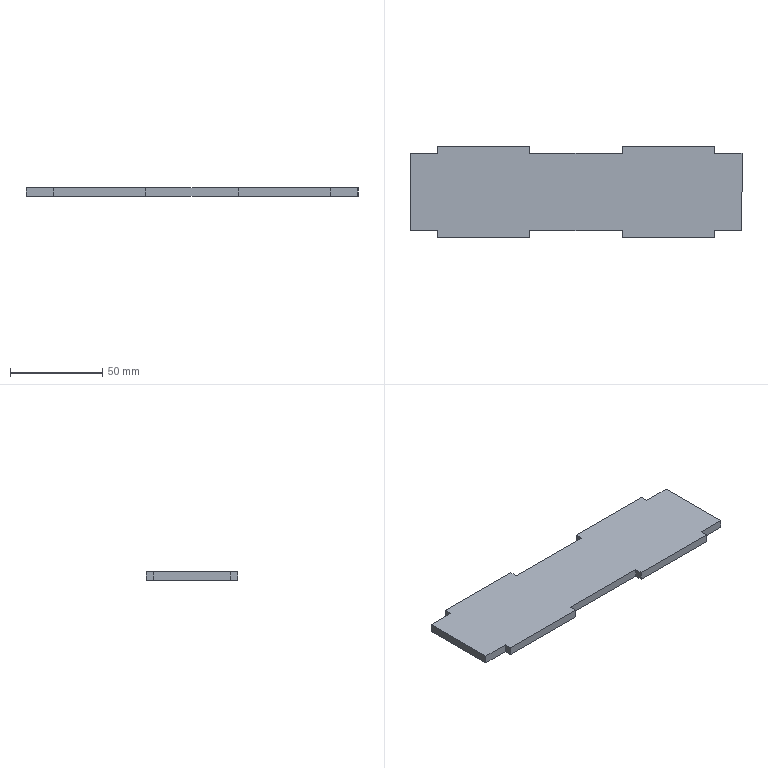Part | SolidWorks | features FlatPattern 1, SMBaseFlange 1, SheetMetal 1 | 1 solid | 22 faces | box 180 x 49.8 x 4.5 mm | volume 37458 mm3 | plane 22
STEP:
#1=CARTESIAN_POINT('',(68.167,-1112.571,0.));
#2=VERTEX_POINT('',#1);
#3=CARTESIAN_POINT('',(53.167,-1112.571,0.));
#4=VERTEX_POINT('',#3);
#5=CARTESIAN_POINT('',(53.167,-1112.571,0.));
#6=DIRECTION('',(-1.,0.,0.));
#7=VECTOR('',#6,1000.);
#8=LINE('',#5,#7);
#9=EDGE_CURVE('',#2,#4,#8,.T.);
#10=ORIENTED_EDGE('',*,*,#9,.F.);
#11=CARTESIAN_POINT('',(68.167,-1112.571,-4.5));
#12=VERTEX_POINT('',#11);
#13=CARTESIAN_POINT('',(68.167,-1112.571,-4.5));
#14=DIRECTION('',(0.,0.,1.));
#15=VECTOR('',#14,1000.);
#16=LINE('',#13,#15);
#17=EDGE_CURVE('',#12,#2,#16,.T.);
#18=ORIENTED_EDGE('',*,*,#17,.F.);
#19=CARTESIAN_POINT('',(53.167,-1112.571,-4.5));
#20=VERTEX_POINT('',#19);
#21=CARTESIAN_POINT('',(53.167,-1112.571,-4.5));
#22=DIRECTION('',(-1.,0.,0.));
#23=VECTOR('',#22,1000.);
#24=LINE('',#21,#23);
#25=EDGE_CURVE('',#12,#20,#24,.T.);
#26=ORIENTED_EDGE('',*,*,#25,.T.);
#27=CARTESIAN_POINT('',(53.167,-1112.571,-4.5));
#28=DIRECTION('',(0.,0.,1.));
#29=VECTOR('',#28,1000.);
#30=LINE('',#27,#29);
#31=EDGE_CURVE('',#20,#4,#30,.T.);
#32=ORIENTED_EDGE('',*,*,#31,.T.);
#33=EDGE_LOOP('',(#10,#18,#26,#32));
#34=FACE_OUTER_BOUND('',#33,.T.);
#35=CARTESIAN_POINT('',(53.167,-1112.571,-4.5));
#36=DIRECTION('',(0.,1.,0.));
#37=DIRECTION('',(0.,0.,1.));
#38=AXIS2_PLACEMENT_3D('',#35,#36,#37);
#39=PLANE('',#38);
#40=ADVANCED_FACE('',(#34),#39,.T.);
#41=CARTESIAN_POINT('',(68.167,-1154.371,0.));
#42=VERTEX_POINT('',#41);
#43=CARTESIAN_POINT('',(68.167,-1112.571,0.));
#44=DIRECTION('',(0.,1.,0.));
#45=VECTOR('',#44,1000.);
#46=LINE('',#43,#45);
#47=EDGE_CURVE('',#42,#2,#46,.T.);
#48=ORIENTED_EDGE('',*,*,#47,.F.);
#49=CARTESIAN_POINT('',(68.167,-1154.371,-4.5));
#50=VERTEX_POINT('',#49);
#51=CARTESIAN_POINT('',(68.167,-1154.371,-4.5));
#52=DIRECTION('',(0.,0.,1.));
#53=VECTOR('',#52,1000.);
#54=LINE('',#51,#53);
#55=EDGE_CURVE('',#50,#42,#54,.T.);
#56=ORIENTED_EDGE('',*,*,#55,.F.);
#57=CARTESIAN_POINT('',(68.167,-1112.571,-4.5));
#58=DIRECTION('',(0.,1.,0.));
#59=VECTOR('',#58,1000.);
#60=LINE('',#57,#59);
#61=EDGE_CURVE('',#50,#12,#60,.T.);
#62=ORIENTED_EDGE('',*,*,#61,.T.);
#63=ORIENTED_EDGE('',*,*,#17,.T.);
#64=EDGE_LOOP('',(#48,#56,#62,#63));
#65=FACE_OUTER_BOUND('',#64,.T.);
#66=CARTESIAN_POINT('',(68.167,-1112.571,-4.5));
#67=DIRECTION('',(1.,0.,0.));
#68=DIRECTION('',(0.,1.,0.));
#69=AXIS2_PLACEMENT_3D('',#66,#67,#68);
#70=PLANE('',#69);
#71=ADVANCED_FACE('',(#65),#70,.T.);
#72=CARTESIAN_POINT('',(53.167,-1154.371,0.));
#73=VERTEX_POINT('',#72);
#74=CARTESIAN_POINT('',(68.167,-1154.371,0.));
#75=DIRECTION('',(1.,0.,0.));
#76=VECTOR('',#75,1000.);
#77=LINE('',#74,#76);
#78=EDGE_CURVE('',#73,#42,#77,.T.);
#79=ORIENTED_EDGE('',*,*,#78,.F.);
#80=CARTESIAN_POINT('',(53.167,-1154.371,-4.5));
#81=VERTEX_POINT('',#80);
#82=CARTESIAN_POINT('',(53.167,-1154.371,-4.5));
#83=DIRECTION('',(0.,0.,1.));
#84=VECTOR('',#83,1000.);
#85=LINE('',#82,#84);
#86=EDGE_CURVE('',#81,#73,#85,.T.);
#87=ORIENTED_EDGE('',*,*,#86,.F.);
#88=CARTESIAN_POINT('',(68.167,-1154.371,-4.5));
#89=DIRECTION('',(1.,0.,0.));
#90=VECTOR('',#89,1000.);
#91=LINE('',#88,#90);
#92=EDGE_CURVE('',#81,#50,#91,.T.);
#93=ORIENTED_EDGE('',*,*,#92,.T.);
#94=ORIENTED_EDGE('',*,*,#55,.T.);
#95=EDGE_LOOP('',(#79,#87,#93,#94));
#96=FACE_OUTER_BOUND('',#95,.T.);
#97=CARTESIAN_POINT('',(68.167,-1154.371,-4.5));
#98=DIRECTION('',(0.,-1.,0.));
#99=DIRECTION('',(0.,0.,-1.));
#100=AXIS2_PLACEMENT_3D('',#97,#98,#99);
#101=PLANE('',#100);
#102=ADVANCED_FACE('',(#96),#101,.T.);
#103=CARTESIAN_POINT('',(53.167,-1158.371,0.));
#104=VERTEX_POINT('',#103);
#105=CARTESIAN_POINT('',(53.167,-1154.371,0.));
#106=DIRECTION('',(0.,1.,0.));
#107=VECTOR('',#106,1000.);
#108=LINE('',#105,#107);
#109=EDGE_CURVE('',#104,#73,#108,.T.);
#110=ORIENTED_EDGE('',*,*,#109,.F.);
#111=CARTESIAN_POINT('',(53.167,-1158.371,-4.5));
#112=VERTEX_POINT('',#111);
#113=CARTESIAN_POINT('',(53.167,-1158.371,-4.5));
#114=DIRECTION('',(0.,0.,1.));
#115=VECTOR('',#114,1000.);
#116=LINE('',#113,#115);
#117=EDGE_CURVE('',#112,#104,#116,.T.);
#118=ORIENTED_EDGE('',*,*,#117,.F.);
#119=CARTESIAN_POINT('',(53.167,-1154.371,-4.5));
#120=DIRECTION('',(0.,1.,0.));
#121=VECTOR('',#120,1000.);
#122=LINE('',#119,#121);
#123=EDGE_CURVE('',#112,#81,#122,.T.);
#124=ORIENTED_EDGE('',*,*,#123,.T.);
#125=ORIENTED_EDGE('',*,*,#86,.T.);
#126=EDGE_LOOP('',(#110,#118,#124,#125));
#127=FACE_OUTER_BOUND('',#126,.T.);
#128=CARTESIAN_POINT('',(53.167,-1154.371,-4.5));
#129=DIRECTION('',(1.,0.,0.));
#130=DIRECTION('',(0.,1.,0.));
#131=AXIS2_PLACEMENT_3D('',#128,#129,#130);
#132=PLANE('',#131);
#133=ADVANCED_FACE('',(#127),#132,.T.);
#134=CARTESIAN_POINT('',(3.167,-1158.371,0.));
#135=VERTEX_POINT('',#134);
#136=CARTESIAN_POINT('',(53.167,-1158.371,0.));
#137=DIRECTION('',(1.,0.,0.));
#138=VECTOR('',#137,1000.);
#139=LINE('',#136,#138);
#140=EDGE_CURVE('',#135,#104,#139,.T.);
#141=ORIENTED_EDGE('',*,*,#140,.F.);
#142=CARTESIAN_POINT('',(3.167,-1158.371,-4.5));
#143=VERTEX_POINT('',#142);
#144=CARTESIAN_POINT('',(3.167,-1158.371,-4.5));
#145=DIRECTION('',(0.,0.,1.));
#146=VECTOR('',#145,1000.);
#147=LINE('',#144,#146);
#148=EDGE_CURVE('',#143,#135,#147,.T.);
#149=ORIENTED_EDGE('',*,*,#148,.F.);
#150=CARTESIAN_POINT('',(53.167,-1158.371,-4.5));
#151=DIRECTION('',(1.,0.,0.));
#152=VECTOR('',#151,1000.);
#153=LINE('',#150,#152);
#154=EDGE_CURVE('',#143,#112,#153,.T.);
#155=ORIENTED_EDGE('',*,*,#154,.T.);
#156=ORIENTED_EDGE('',*,*,#117,.T.);
#157=EDGE_LOOP('',(#141,#149,#155,#156));
#158=FACE_OUTER_BOUND('',#157,.T.);
#159=CARTESIAN_POINT('',(53.167,-1158.371,-4.5));
#160=DIRECTION('',(0.,-1.,0.));
#161=DIRECTION('',(0.,0.,-1.));
#162=AXIS2_PLACEMENT_3D('',#159,#160,#161);
#163=PLANE('',#162);
#164=ADVANCED_FACE('',(#158),#163,.T.);
#165=CARTESIAN_POINT('',(3.167,-1154.371,0.));
#166=VERTEX_POINT('',#165);
#167=CARTESIAN_POINT('',(3.167,-1158.371,0.));
#168=DIRECTION('',(0.,-1.,0.));
#169=VECTOR('',#168,1000.);
#170=LINE('',#167,#169);
#171=EDGE_CURVE('',#166,#135,#170,.T.);
#172=ORIENTED_EDGE('',*,*,#171,.F.);
#173=CARTESIAN_POINT('',(3.167,-1154.371,-4.5));
#174=VERTEX_POINT('',#173);
#175=CARTESIAN_POINT('',(3.167,-1154.371,-4.5));
#176=DIRECTION('',(0.,0.,1.));
#177=VECTOR('',#176,1000.);
#178=LINE('',#175,#177);
#179=EDGE_CURVE('',#174,#166,#178,.T.);
#180=ORIENTED_EDGE('',*,*,#179,.F.);
#181=CARTESIAN_POINT('',(3.167,-1158.371,-4.5));
#182=DIRECTION('',(0.,-1.,0.));
#183=VECTOR('',#182,1000.);
#184=LINE('',#181,#183);
#185=EDGE_CURVE('',#174,#143,#184,.T.);
#186=ORIENTED_EDGE('',*,*,#185,.T.);
#187=ORIENTED_EDGE('',*,*,#148,.T.);
#188=EDGE_LOOP('',(#172,#180,#186,#187));
#189=FACE_OUTER_BOUND('',#188,.T.);
#190=CARTESIAN_POINT('',(3.167,-1158.371,-4.5));
#191=DIRECTION('',(-1.,0.,0.));
#192=DIRECTION('',(0.,-1.,0.));
#193=AXIS2_PLACEMENT_3D('',#190,#191,#192);
#194=PLANE('',#193);
#195=ADVANCED_FACE('',(#189),#194,.T.);
#196=CARTESIAN_POINT('',(-46.833,-1154.371,0.));
#197=VERTEX_POINT('',#196);
#198=CARTESIAN_POINT('',(3.167,-1154.371,0.));
#199=DIRECTION('',(1.,0.,0.));
#200=VECTOR('',#199,1000.);
#201=LINE('',#198,#200);
#202=EDGE_CURVE('',#197,#166,#201,.T.);
#203=ORIENTED_EDGE('',*,*,#202,.F.);
#204=CARTESIAN_POINT('',(-46.833,-1154.371,-4.5));
#205=VERTEX_POINT('',#204);
#206=CARTESIAN_POINT('',(-46.833,-1154.371,-4.5));
#207=DIRECTION('',(0.,0.,1.));
#208=VECTOR('',#207,1000.);
#209=LINE('',#206,#208);
#210=EDGE_CURVE('',#205,#197,#209,.T.);
#211=ORIENTED_EDGE('',*,*,#210,.F.);
#212=CARTESIAN_POINT('',(3.167,-1154.371,-4.5));
#213=DIRECTION('',(1.,0.,0.));
#214=VECTOR('',#213,1000.);
#215=LINE('',#212,#214);
#216=EDGE_CURVE('',#205,#174,#215,.T.);
#217=ORIENTED_EDGE('',*,*,#216,.T.);
#218=ORIENTED_EDGE('',*,*,#179,.T.);
#219=EDGE_LOOP('',(#203,#211,#217,#218));
#220=FACE_OUTER_BOUND('',#219,.T.);
#221=CARTESIAN_POINT('',(3.167,-1154.371,-4.5));
#222=DIRECTION('',(0.,-1.,0.));
#223=DIRECTION('',(0.,0.,-1.));
#224=AXIS2_PLACEMENT_3D('',#221,#222,#223);
#225=PLANE('',#224);
#226=ADVANCED_FACE('',(#220),#225,.T.);
#227=CARTESIAN_POINT('',(-46.833,-1158.371,0.));
#228=VERTEX_POINT('',#227);
#229=CARTESIAN_POINT('',(-46.833,-1154.371,0.));
#230=DIRECTION('',(0.,1.,0.));
#231=VECTOR('',#230,1000.);
#232=LINE('',#229,#231);
#233=EDGE_CURVE('',#228,#197,#232,.T.);
#234=ORIENTED_EDGE('',*,*,#233,.F.);
#235=CARTESIAN_POINT('',(-46.833,-1158.371,-4.5));
#236=VERTEX_POINT('',#235);
#237=CARTESIAN_POINT('',(-46.833,-1158.371,-4.5));
#238=DIRECTION('',(0.,0.,1.));
#239=VECTOR('',#238,1000.);
#240=LINE('',#237,#239);
#241=EDGE_CURVE('',#236,#228,#240,.T.);
#242=ORIENTED_EDGE('',*,*,#241,.F.);
#243=CARTESIAN_POINT('',(-46.833,-1154.371,-4.5));
#244=DIRECTION('',(0.,1.,0.));
#245=VECTOR('',#244,1000.);
#246=LINE('',#243,#245);
#247=EDGE_CURVE('',#236,#205,#246,.T.);
#248=ORIENTED_EDGE('',*,*,#247,.T.);
#249=ORIENTED_EDGE('',*,*,#210,.T.);
#250=EDGE_LOOP('',(#234,#242,#248,#249));
#251=FACE_OUTER_BOUND('',#250,.T.);
#252=CARTESIAN_POINT('',(-46.833,-1154.371,-4.5));
#253=DIRECTION('',(1.,0.,0.));
#254=DIRECTION('',(0.,0.,-1.));
#255=AXIS2_PLACEMENT_3D('',#252,#253,#254);
#256=PLANE('',#255);
#257=ADVANCED_FACE('',(#251),#256,.T.);
#258=CARTESIAN_POINT('',(-96.833,-1158.371,0.));
#259=VERTEX_POINT('',#258);
#260=CARTESIAN_POINT('',(-46.833,-1158.371,0.));
#261=DIRECTION('',(1.,0.,0.));
#262=VECTOR('',#261,1000.);
#263=LINE('',#260,#262);
#264=EDGE_CURVE('',#259,#228,#263,.T.);
#265=ORIENTED_EDGE('',*,*,#264,.F.);
#266=CARTESIAN_POINT('',(-96.833,-1158.371,-4.5));
#267=VERTEX_POINT('',#266);
#268=CARTESIAN_POINT('',(-96.833,-1158.371,-4.5));
#269=DIRECTION('',(0.,0.,1.));
#270=VECTOR('',#269,1000.);
#271=LINE('',#268,#270);
#272=EDGE_CURVE('',#267,#259,#271,.T.);
#273=ORIENTED_EDGE('',*,*,#272,.F.);
#274=CARTESIAN_POINT('',(-46.833,-1158.371,-4.5));
#275=DIRECTION('',(1.,0.,0.));
#276=VECTOR('',#275,1000.);
#277=LINE('',#274,#276);
#278=EDGE_CURVE('',#267,#236,#277,.T.);
#279=ORIENTED_EDGE('',*,*,#278,.T.);
#280=ORIENTED_EDGE('',*,*,#241,.T.);
#281=EDGE_LOOP('',(#265,#273,#279,#280));
#282=FACE_OUTER_BOUND('',#281,.T.);
#283=CARTESIAN_POINT('',(-46.833,-1158.371,-4.5));
#284=DIRECTION('',(0.,-1.,0.));
#285=DIRECTION('',(0.,0.,-1.));
#286=AXIS2_PLACEMENT_3D('',#283,#284,#285);
#287=PLANE('',#286);
#288=ADVANCED_FACE('',(#282),#287,.T.);
#289=CARTESIAN_POINT('',(-96.833,-1154.371,0.));
#290=VERTEX_POINT('',#289);
#291=CARTESIAN_POINT('',(-96.833,-1158.371,0.));
#292=DIRECTION('',(0.,-1.,0.));
#293=VECTOR('',#292,1000.);
#294=LINE('',#291,#293);
#295=EDGE_CURVE('',#290,#259,#294,.T.);
#296=ORIENTED_EDGE('',*,*,#295,.F.);
#297=CARTESIAN_POINT('',(-96.833,-1154.371,-4.5));
#298=VERTEX_POINT('',#297);
#299=CARTESIAN_POINT('',(-96.833,-1154.371,-4.5));
#300=DIRECTION('',(0.,0.,1.));
#301=VECTOR('',#300,1000.);
#302=LINE('',#299,#301);
#303=EDGE_CURVE('',#298,#290,#302,.T.);
#304=ORIENTED_EDGE('',*,*,#303,.F.);
#305=CARTESIAN_POINT('',(-96.833,-1158.371,-4.5));
#306=DIRECTION('',(0.,-1.,0.));
#307=VECTOR('',#306,1000.);
#308=LINE('',#305,#307);
#309=EDGE_CURVE('',#298,#267,#308,.T.);
#310=ORIENTED_EDGE('',*,*,#309,.T.);
#311=ORIENTED_EDGE('',*,*,#272,.T.);
#312=EDGE_LOOP('',(#296,#304,#310,#311));
#313=FACE_OUTER_BOUND('',#312,.T.);
#314=CARTESIAN_POINT('',(-96.833,-1158.371,-4.5));
#315=DIRECTION('',(-1.,0.,0.));
#316=DIRECTION('',(0.,0.,1.));
#317=AXIS2_PLACEMENT_3D('',#314,#315,#316);
#318=PLANE('',#317);
#319=ADVANCED_FACE('',(#313),#318,.T.);
#320=CARTESIAN_POINT('',(-111.833,-1154.371,0.));
#321=VERTEX_POINT('',#320);
#322=CARTESIAN_POINT('',(-96.833,-1154.371,0.));
#323=DIRECTION('',(1.,0.,0.));
#324=VECTOR('',#323,1000.);
#325=LINE('',#322,#324);
#326=EDGE_CURVE('',#321,#290,#325,.T.);
#327=ORIENTED_EDGE('',*,*,#326,.F.);
#328=CARTESIAN_POINT('',(-111.833,-1154.371,-4.5));
#329=VERTEX_POINT('',#328);
#330=CARTESIAN_POINT('',(-111.833,-1154.371,-4.5));
#331=DIRECTION('',(0.,0.,1.));
#332=VECTOR('',#331,1000.);
#333=LINE('',#330,#332);
#334=EDGE_CURVE('',#329,#321,#333,.T.);
#335=ORIENTED_EDGE('',*,*,#334,.F.);
#336=CARTESIAN_POINT('',(-96.833,-1154.371,-4.5));
#337=DIRECTION('',(1.,0.,0.));
#338=VECTOR('',#337,1000.);
#339=LINE('',#336,#338);
#340=EDGE_CURVE('',#329,#298,#339,.T.);
#341=ORIENTED_EDGE('',*,*,#340,.T.);
#342=ORIENTED_EDGE('',*,*,#303,.T.);
#343=EDGE_LOOP('',(#327,#335,#341,#342));
#344=FACE_OUTER_BOUND('',#343,.T.);
#345=CARTESIAN_POINT('',(-96.833,-1154.371,-4.5));
#346=DIRECTION('',(0.,-1.,0.));
#347=DIRECTION('',(0.,0.,-1.));
#348=AXIS2_PLACEMENT_3D('',#345,#346,#347);
#349=PLANE('',#348);
#350=ADVANCED_FACE('',(#344),#349,.T.);
#351=CARTESIAN_POINT('',(-111.833,-1112.571,0.));
#352=VERTEX_POINT('',#351);
#353=CARTESIAN_POINT('',(-111.833,-1154.371,0.));
#354=DIRECTION('',(0.,-1.,0.));
#355=VECTOR('',#354,1000.);
#356=LINE('',#353,#355);
#357=EDGE_CURVE('',#352,#321,#356,.T.);
#358=ORIENTED_EDGE('',*,*,#357,.F.);
#359=CARTESIAN_POINT('',(-111.833,-1112.571,-4.5));
#360=VERTEX_POINT('',#359);
#361=CARTESIAN_POINT('',(-111.833,-1112.571,-4.5));
#362=DIRECTION('',(0.,0.,1.));
#363=VECTOR('',#362,1000.);
#364=LINE('',#361,#363);
#365=EDGE_CURVE('',#360,#352,#364,.T.);
#366=ORIENTED_EDGE('',*,*,#365,.F.);
#367=CARTESIAN_POINT('',(-111.833,-1154.371,-4.5));
#368=DIRECTION('',(0.,-1.,0.));
#369=VECTOR('',#368,1000.);
#370=LINE('',#367,#369);
#371=EDGE_CURVE('',#360,#329,#370,.T.);
#372=ORIENTED_EDGE('',*,*,#371,.T.);
#373=ORIENTED_EDGE('',*,*,#334,.T.);
#374=EDGE_LOOP('',(#358,#366,#372,#373));
#375=FACE_OUTER_BOUND('',#374,.T.);
#376=CARTESIAN_POINT('',(-111.833,-1154.371,-4.5));
#377=DIRECTION('',(-1.,0.,0.));
#378=DIRECTION('',(0.,-1.,0.));
#379=AXIS2_PLACEMENT_3D('',#376,#377,#378);
#380=PLANE('',#379);
#381=ADVANCED_FACE('',(#375),#380,.T.);
#382=CARTESIAN_POINT('',(-96.833,-1112.571,0.));
#383=VERTEX_POINT('',#382);
#384=CARTESIAN_POINT('',(-111.833,-1112.571,0.));
#385=DIRECTION('',(-1.,0.,0.));
#386=VECTOR('',#385,1000.);
#387=LINE('',#384,#386);
#388=EDGE_CURVE('',#383,#352,#387,.T.);
#389=ORIENTED_EDGE('',*,*,#388,.F.);
#390=CARTESIAN_POINT('',(-96.833,-1112.571,-4.5));
#391=VERTEX_POINT('',#390);
#392=CARTESIAN_POINT('',(-96.833,-1112.571,-4.5));
#393=DIRECTION('',(0.,0.,1.));
#394=VECTOR('',#393,1000.);
#395=LINE('',#392,#394);
#396=EDGE_CURVE('',#391,#383,#395,.T.);
#397=ORIENTED_EDGE('',*,*,#396,.F.);
#398=CARTESIAN_POINT('',(-111.833,-1112.571,-4.5));
#399=DIRECTION('',(-1.,0.,0.));
#400=VECTOR('',#399,1000.);
#401=LINE('',#398,#400);
#402=EDGE_CURVE('',#391,#360,#401,.T.);
#403=ORIENTED_EDGE('',*,*,#402,.T.);
#404=ORIENTED_EDGE('',*,*,#365,.T.);
#405=EDGE_LOOP('',(#389,#397,#403,#404));
#406=FACE_OUTER_BOUND('',#405,.T.);
#407=CARTESIAN_POINT('',(-111.833,-1112.571,-4.5));
#408=DIRECTION('',(0.,1.,0.));
#409=DIRECTION('',(0.,0.,1.));
#410=AXIS2_PLACEMENT_3D('',#407,#408,#409);
#411=PLANE('',#410);
#412=ADVANCED_FACE('',(#406),#411,.T.);
#413=CARTESIAN_POINT('',(-96.833,-1108.571,0.));
#414=VERTEX_POINT('',#413);
#415=CARTESIAN_POINT('',(-96.833,-1112.571,0.));
#416=DIRECTION('',(0.,-1.,0.));
#417=VECTOR('',#416,1000.);
#418=LINE('',#415,#417);
#419=EDGE_CURVE('',#414,#383,#418,.T.);
#420=ORIENTED_EDGE('',*,*,#419,.F.);
#421=CARTESIAN_POINT('',(-96.833,-1108.571,-4.5));
#422=VERTEX_POINT('',#421);
#423=CARTESIAN_POINT('',(-96.833,-1108.571,-4.5));
#424=DIRECTION('',(0.,0.,1.));
#425=VECTOR('',#424,1000.);
#426=LINE('',#423,#425);
#427=EDGE_CURVE('',#422,#414,#426,.T.);
#428=ORIENTED_EDGE('',*,*,#427,.F.);
#429=CARTESIAN_POINT('',(-96.833,-1112.571,-4.5));
#430=DIRECTION('',(0.,-1.,0.));
#431=VECTOR('',#430,1000.);
#432=LINE('',#429,#431);
#433=EDGE_CURVE('',#422,#391,#432,.T.);
#434=ORIENTED_EDGE('',*,*,#433,.T.);
#435=ORIENTED_EDGE('',*,*,#396,.T.);
#436=EDGE_LOOP('',(#420,#428,#434,#435));
#437=FACE_OUTER_BOUND('',#436,.T.);
#438=CARTESIAN_POINT('',(-96.833,-1112.571,-4.5));
#439=DIRECTION('',(-1.,0.,0.));
#440=DIRECTION('',(0.,-1.,0.));
#441=AXIS2_PLACEMENT_3D('',#438,#439,#440);
#442=PLANE('',#441);
#443=ADVANCED_FACE('',(#437),#442,.T.);
#444=CARTESIAN_POINT('',(-46.833,-1108.571,0.));
#445=VERTEX_POINT('',#444);
#446=CARTESIAN_POINT('',(-96.833,-1108.571,0.));
#447=DIRECTION('',(-1.,0.,0.));
#448=VECTOR('',#447,1000.);
#449=LINE('',#446,#448);
#450=EDGE_CURVE('',#445,#414,#449,.T.);
#451=ORIENTED_EDGE('',*,*,#450,.F.);
#452=CARTESIAN_POINT('',(-46.833,-1108.571,-4.5));
#453=VERTEX_POINT('',#452);
#454=CARTESIAN_POINT('',(-46.833,-1108.571,-4.5));
#455=DIRECTION('',(0.,0.,1.));
#456=VECTOR('',#455,1000.);
#457=LINE('',#454,#456);
#458=EDGE_CURVE('',#453,#445,#457,.T.);
#459=ORIENTED_EDGE('',*,*,#458,.F.);
#460=CARTESIAN_POINT('',(-96.833,-1108.571,-4.5));
#461=DIRECTION('',(-1.,0.,0.));
#462=VECTOR('',#461,1000.);
#463=LINE('',#460,#462);
#464=EDGE_CURVE('',#453,#422,#463,.T.);
#465=ORIENTED_EDGE('',*,*,#464,.T.);
#466=ORIENTED_EDGE('',*,*,#427,.T.);
#467=EDGE_LOOP('',(#451,#459,#465,#466));
#468=FACE_OUTER_BOUND('',#467,.T.);
#469=CARTESIAN_POINT('',(-96.833,-1108.571,-4.5));
#470=DIRECTION('',(0.,1.,0.));
#471=DIRECTION('',(0.,0.,1.));
#472=AXIS2_PLACEMENT_3D('',#469,#470,#471);
#473=PLANE('',#472);
#474=ADVANCED_FACE('',(#468),#473,.T.);
#475=CARTESIAN_POINT('',(-46.833,-1112.571,0.));
#476=VERTEX_POINT('',#475);
#477=CARTESIAN_POINT('',(-46.833,-1108.571,0.));
#478=DIRECTION('',(0.,1.,0.));
#479=VECTOR('',#478,1000.);
#480=LINE('',#477,#479);
#481=EDGE_CURVE('',#476,#445,#480,.T.);
#482=ORIENTED_EDGE('',*,*,#481,.F.);
#483=CARTESIAN_POINT('',(-46.833,-1112.571,-4.5));
#484=VERTEX_POINT('',#483);
#485=CARTESIAN_POINT('',(-46.833,-1112.571,-4.5));
#486=DIRECTION('',(0.,0.,1.));
#487=VECTOR('',#486,1000.);
#488=LINE('',#485,#487);
#489=EDGE_CURVE('',#484,#476,#488,.T.);
#490=ORIENTED_EDGE('',*,*,#489,.F.);
#491=CARTESIAN_POINT('',(-46.833,-1108.571,-4.5));
#492=DIRECTION('',(0.,1.,0.));
#493=VECTOR('',#492,1000.);
#494=LINE('',#491,#493);
#495=EDGE_CURVE('',#484,#453,#494,.T.);
#496=ORIENTED_EDGE('',*,*,#495,.T.);
#497=ORIENTED_EDGE('',*,*,#458,.T.);
#498=EDGE_LOOP('',(#482,#490,#496,#497));
#499=FACE_OUTER_BOUND('',#498,.T.);
#500=CARTESIAN_POINT('',(-46.833,-1108.571,-4.5));
#501=DIRECTION('',(1.,0.,0.));
#502=DIRECTION('',(0.,1.,0.));
#503=AXIS2_PLACEMENT_3D('',#500,#501,#502);
#504=PLANE('',#503);
#505=ADVANCED_FACE('',(#499),#504,.T.);
#506=CARTESIAN_POINT('',(3.167,-1112.571,0.));
#507=VERTEX_POINT('',#506);
#508=CARTESIAN_POINT('',(-46.833,-1112.571,0.));
#509=DIRECTION('',(-1.,0.,0.));
#510=VECTOR('',#509,1000.);
#511=LINE('',#508,#510);
#512=EDGE_CURVE('',#507,#476,#511,.T.);
#513=ORIENTED_EDGE('',*,*,#512,.F.);
#514=CARTESIAN_POINT('',(3.167,-1112.571,-4.5));
#515=VERTEX_POINT('',#514);
#516=CARTESIAN_POINT('',(3.167,-1112.571,-4.5));
#517=DIRECTION('',(0.,0.,1.));
#518=VECTOR('',#517,1000.);
#519=LINE('',#516,#518);
#520=EDGE_CURVE('',#515,#507,#519,.T.);
#521=ORIENTED_EDGE('',*,*,#520,.F.);
#522=CARTESIAN_POINT('',(-46.833,-1112.571,-4.5));
#523=DIRECTION('',(-1.,0.,0.));
#524=VECTOR('',#523,1000.);
#525=LINE('',#522,#524);
#526=EDGE_CURVE('',#515,#484,#525,.T.);
#527=ORIENTED_EDGE('',*,*,#526,.T.);
#528=ORIENTED_EDGE('',*,*,#489,.T.);
#529=EDGE_LOOP('',(#513,#521,#527,#528));
#530=FACE_OUTER_BOUND('',#529,.T.);
#531=CARTESIAN_POINT('',(-46.833,-1112.571,-4.5));
#532=DIRECTION('',(0.,1.,0.));
#533=DIRECTION('',(0.,0.,1.));
#534=AXIS2_PLACEMENT_3D('',#531,#532,#533);
#535=PLANE('',#534);
#536=ADVANCED_FACE('',(#530),#535,.T.);
#537=CARTESIAN_POINT('',(3.167,-1108.571,0.));
#538=VERTEX_POINT('',#537);
#539=CARTESIAN_POINT('',(3.167,-1108.571,0.));
#540=DIRECTION('',(0.,-1.,0.));
#541=VECTOR('',#540,1000.);
#542=LINE('',#539,#541);
#543=EDGE_CURVE('',#538,#507,#542,.T.);
#544=ORIENTED_EDGE('',*,*,#543,.F.);
#545=CARTESIAN_POINT('',(3.167,-1108.571,-4.5));
#546=VERTEX_POINT('',#545);
#547=CARTESIAN_POINT('',(3.167,-1108.571,-4.5));
#548=DIRECTION('',(0.,0.,1.));
#549=VECTOR('',#548,1000.);
#550=LINE('',#547,#549);
#551=EDGE_CURVE('',#546,#538,#550,.T.);
#552=ORIENTED_EDGE('',*,*,#551,.F.);
#553=CARTESIAN_POINT('',(3.167,-1108.571,-4.5));
#554=DIRECTION('',(0.,-1.,0.));
#555=VECTOR('',#554,1000.);
#556=LINE('',#553,#555);
#557=EDGE_CURVE('',#546,#515,#556,.T.);
#558=ORIENTED_EDGE('',*,*,#557,.T.);
#559=ORIENTED_EDGE('',*,*,#520,.T.);
#560=EDGE_LOOP('',(#544,#552,#558,#559));
#561=FACE_OUTER_BOUND('',#560,.T.);
#562=CARTESIAN_POINT('',(3.167,-1108.571,-4.5));
#563=DIRECTION('',(-1.,0.,0.));
#564=DIRECTION('',(0.,-1.,0.));
#565=AXIS2_PLACEMENT_3D('',#562,#563,#564);
#566=PLANE('',#565);
#567=ADVANCED_FACE('',(#561),#566,.T.);
#568=CARTESIAN_POINT('',(53.167,-1108.571,0.));
#569=VERTEX_POINT('',#568);
#570=CARTESIAN_POINT('',(53.167,-1108.571,0.));
#571=DIRECTION('',(-1.,0.,0.));
#572=VECTOR('',#571,1000.);
#573=LINE('',#570,#572);
#574=EDGE_CURVE('',#569,#538,#573,.T.);
#575=ORIENTED_EDGE('',*,*,#574,.F.);
#576=CARTESIAN_POINT('',(53.167,-1108.571,-4.5));
#577=VERTEX_POINT('',#576);
#578=CARTESIAN_POINT('',(53.167,-1108.571,-4.5));
#579=DIRECTION('',(0.,0.,1.));
#580=VECTOR('',#579,1000.);
#581=LINE('',#578,#580);
#582=EDGE_CURVE('',#577,#569,#581,.T.);
#583=ORIENTED_EDGE('',*,*,#582,.F.);
#584=CARTESIAN_POINT('',(53.167,-1108.571,-4.5));
#585=DIRECTION('',(-1.,0.,0.));
#586=VECTOR('',#585,1000.);
#587=LINE('',#584,#586);
#588=EDGE_CURVE('',#577,#546,#587,.T.);
#589=ORIENTED_EDGE('',*,*,#588,.T.);
#590=ORIENTED_EDGE('',*,*,#551,.T.);
#591=EDGE_LOOP('',(#575,#583,#589,#590));
#592=FACE_OUTER_BOUND('',#591,.T.);
#593=CARTESIAN_POINT('',(53.167,-1108.571,-4.5));
#594=DIRECTION('',(0.,1.,0.));
#595=DIRECTION('',(0.,0.,1.));
#596=AXIS2_PLACEMENT_3D('',#593,#594,#595);
#597=PLANE('',#596);
#598=ADVANCED_FACE('',(#592),#597,.T.);
#599=CARTESIAN_POINT('',(53.167,-1112.571,0.));
#600=DIRECTION('',(0.,1.,0.));
#601=VECTOR('',#600,1000.);
#602=LINE('',#599,#601);
#603=EDGE_CURVE('',#4,#569,#602,.T.);
#604=ORIENTED_EDGE('',*,*,#603,.F.);
#605=ORIENTED_EDGE('',*,*,#31,.F.);
#606=CARTESIAN_POINT('',(53.167,-1112.571,-4.5));
#607=DIRECTION('',(0.,1.,0.));
#608=VECTOR('',#607,1000.);
#609=LINE('',#606,#608);
#610=EDGE_CURVE('',#20,#577,#609,.T.);
#611=ORIENTED_EDGE('',*,*,#610,.T.);
#612=ORIENTED_EDGE('',*,*,#582,.T.);
#613=EDGE_LOOP('',(#604,#605,#611,#612));
#614=FACE_OUTER_BOUND('',#613,.T.);
#615=CARTESIAN_POINT('',(53.167,-1112.571,-4.5));
#616=DIRECTION('',(1.,0.,0.));
#617=DIRECTION('',(0.,0.,-1.));
#618=AXIS2_PLACEMENT_3D('',#615,#616,#617);
#619=PLANE('',#618);
#620=ADVANCED_FACE('',(#614),#619,.T.);
#621=ORIENTED_EDGE('',*,*,#25,.F.);
#622=ORIENTED_EDGE('',*,*,#61,.F.);
#623=ORIENTED_EDGE('',*,*,#92,.F.);
#624=ORIENTED_EDGE('',*,*,#123,.F.);
#625=ORIENTED_EDGE('',*,*,#154,.F.);
#626=ORIENTED_EDGE('',*,*,#185,.F.);
#627=ORIENTED_EDGE('',*,*,#216,.F.);
#628=ORIENTED_EDGE('',*,*,#247,.F.);
#629=ORIENTED_EDGE('',*,*,#278,.F.);
#630=ORIENTED_EDGE('',*,*,#309,.F.);
#631=ORIENTED_EDGE('',*,*,#340,.F.);
#632=ORIENTED_EDGE('',*,*,#371,.F.);
#633=ORIENTED_EDGE('',*,*,#402,.F.);
#634=ORIENTED_EDGE('',*,*,#433,.F.);
#635=ORIENTED_EDGE('',*,*,#464,.F.);
#636=ORIENTED_EDGE('',*,*,#495,.F.);
#637=ORIENTED_EDGE('',*,*,#526,.F.);
#638=ORIENTED_EDGE('',*,*,#557,.F.);
#639=ORIENTED_EDGE('',*,*,#588,.F.);
#640=ORIENTED_EDGE('',*,*,#610,.F.);
#641=EDGE_LOOP('',(#621,#622,#623,#624,#625,#626,#627,#628,#629,#630,#631,#632,#633,#634,#635,#636,#637,#638,#639,#640));
#642=FACE_OUTER_BOUND('',#641,.T.);
#643=CARTESIAN_POINT('',(0.,0.,-4.5));
#644=DIRECTION('',(0.,0.,-1.));
#645=DIRECTION('',(-1.,0.,0.));
#646=AXIS2_PLACEMENT_3D('',#643,#644,#645);
#647=PLANE('',#646);
#648=ADVANCED_FACE('',(#642),#647,.T.);
#649=ORIENTED_EDGE('',*,*,#9,.T.);
#650=ORIENTED_EDGE('',*,*,#603,.T.);
#651=ORIENTED_EDGE('',*,*,#574,.T.);
#652=ORIENTED_EDGE('',*,*,#543,.T.);
#653=ORIENTED_EDGE('',*,*,#512,.T.);
#654=ORIENTED_EDGE('',*,*,#481,.T.);
#655=ORIENTED_EDGE('',*,*,#450,.T.);
#656=ORIENTED_EDGE('',*,*,#419,.T.);
#657=ORIENTED_EDGE('',*,*,#388,.T.);
#658=ORIENTED_EDGE('',*,*,#357,.T.);
#659=ORIENTED_EDGE('',*,*,#326,.T.);
#660=ORIENTED_EDGE('',*,*,#295,.T.);
#661=ORIENTED_EDGE('',*,*,#264,.T.);
#662=ORIENTED_EDGE('',*,*,#233,.T.);
#663=ORIENTED_EDGE('',*,*,#202,.T.);
#664=ORIENTED_EDGE('',*,*,#171,.T.);
#665=ORIENTED_EDGE('',*,*,#140,.T.);
#666=ORIENTED_EDGE('',*,*,#109,.T.);
#667=ORIENTED_EDGE('',*,*,#78,.T.);
#668=ORIENTED_EDGE('',*,*,#47,.T.);
#669=EDGE_LOOP('',(#649,#650,#651,#652,#653,#654,#655,#656,#657,#658,#659,#660,#661,#662,#663,#664,#665,#666,#667,#668));
#670=FACE_OUTER_BOUND('',#669,.T.);
#671=CARTESIAN_POINT('',(0.,0.,0.));
#672=DIRECTION('',(0.,0.,-1.));
#673=DIRECTION('',(-1.,0.,0.));
#674=AXIS2_PLACEMENT_3D('',#671,#672,#673);
#675=PLANE('',#674);
#676=ADVANCED_FACE('',(#670),#675,.F.);
#677=CLOSED_SHELL('',(#40,#71,#102,#133,#164,#195,#226,#257,#288,#319,#350,#381,#412,#443,#474,#505,#536,#567,#598,#620,#648,#676));
#678=MANIFOLD_SOLID_BREP('',#677);
#679=CARTESIAN_POINT('',(0.,0.,0.));
#680=DIRECTION('',(0.,0.,1.));
#681=DIRECTION('',(1.,0.,0.));
#682=AXIS2_PLACEMENT_3D('',#679,#680,#681);
#683=(LENGTH_UNIT()NAMED_UNIT(*)SI_UNIT(.MILLI.,.METRE.));
#684=UNCERTAINTY_MEASURE_WITH_UNIT(LENGTH_MEASURE(0.00001),#683,'','');
#685=(NAMED_UNIT(*)PLANE_ANGLE_UNIT()SI_UNIT($,.RADIAN.));
#686=(NAMED_UNIT(*)SI_UNIT($,.STERADIAN.)SOLID_ANGLE_UNIT());
#687=(GEOMETRIC_REPRESENTATION_CONTEXT(3)GLOBAL_UNCERTAINTY_ASSIGNED_CONTEXT((#684))GLOBAL_UNIT_ASSIGNED_CONTEXT((#683,#685,#686))REPRESENTATION_CONTEXT('',''));
#688=ADVANCED_BREP_SHAPE_REPRESENTATION('',(#678,#682),#687);